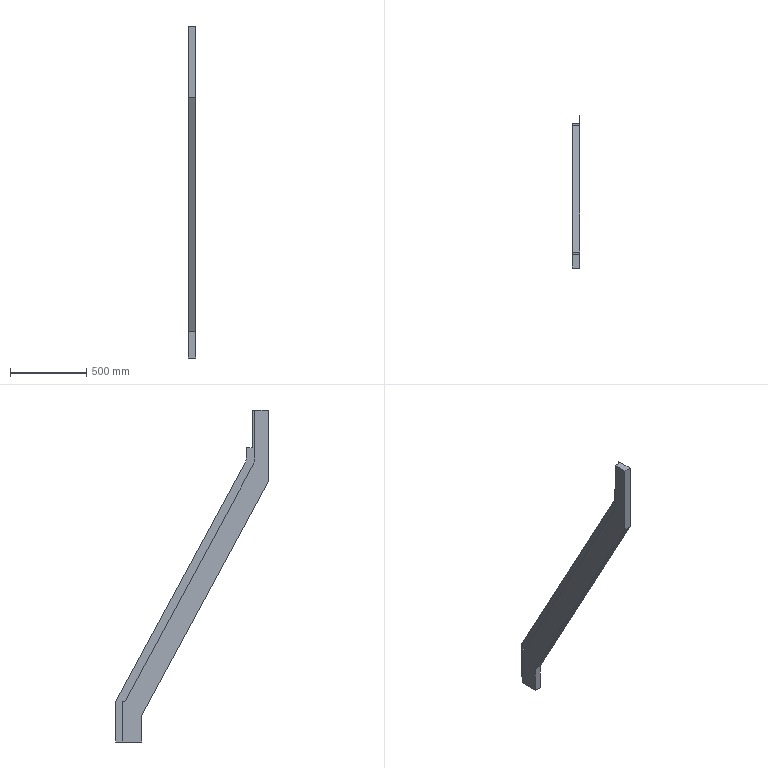Part | NX | 1 solid | 19 faces | box 48 x 1000 x 2173 mm | volume 15101075 mm3 | plane 17 | cylinder 2 | commonest cylinder face diameters 120 x1 228 x1
STEP:
#1=CARTESIAN_POINT('',(38.874,311.682,323.798));
#2=VERTEX_POINT('',#1);
#3=CARTESIAN_POINT('',(38.874,311.682,589.52));
#4=VERTEX_POINT('',#3);
#5=CARTESIAN_POINT('',(38.874,311.682,323.798));
#6=DIRECTION('',(0.,0.,1.));
#7=VECTOR('',#6,1.);
#8=LINE('',#5,#7);
#9=EDGE_CURVE('',#2,#4,#8,.T.);
#10=ORIENTED_EDGE('',*,*,#9,.T.);
#11=CARTESIAN_POINT('',(40.674,311.682,589.52));
#12=VERTEX_POINT('',#11);
#13=CARTESIAN_POINT('',(38.874,311.682,589.52));
#14=DIRECTION('',(1.,0.,0.));
#15=VECTOR('',#14,1.);
#16=LINE('',#13,#15);
#17=EDGE_CURVE('',#4,#12,#16,.T.);
#18=ORIENTED_EDGE('',*,*,#17,.T.);
#19=CARTESIAN_POINT('',(40.674,311.682,323.798));
#20=VERTEX_POINT('',#19);
#21=CARTESIAN_POINT('',(40.674,311.682,323.798));
#22=DIRECTION('',(0.,0.,1.));
#23=VECTOR('',#22,1.);
#24=LINE('',#21,#23);
#25=EDGE_CURVE('',#20,#12,#24,.T.);
#26=ORIENTED_EDGE('',*,*,#25,.F.);
#27=CARTESIAN_POINT('',(40.674,311.682,323.798));
#28=DIRECTION('',(-1.,0.,0.));
#29=VECTOR('',#28,1.);
#30=LINE('',#27,#29);
#31=EDGE_CURVE('',#20,#2,#30,.T.);
#32=ORIENTED_EDGE('',*,*,#31,.T.);
#33=EDGE_LOOP('',(#10,#18,#26,#32));
#34=FACE_OUTER_BOUND('',#33,.T.);
#35=CARTESIAN_POINT('',(40.674,311.682,323.798));
#36=DIRECTION('',(0.,1.,0.));
#37=DIRECTION('',(0.,0.,1.));
#38=AXIS2_PLACEMENT_3D('',#35,#36,#37);
#39=PLANE('',#38);
#40=ADVANCED_FACE('',(#34),#39,.T.);
#41=CARTESIAN_POINT('',(40.674,-583.499,2251.086));
#42=VERTEX_POINT('',#41);
#43=CARTESIAN_POINT('',(40.674,-544.499,2251.086));
#44=VERTEX_POINT('',#43);
#45=CARTESIAN_POINT('',(40.674,-544.499,2251.086));
#46=DIRECTION('',(0.,1.,0.));
#47=VECTOR('',#46,1.);
#48=LINE('',#45,#47);
#49=EDGE_CURVE('',#42,#44,#48,.T.);
#50=ORIENTED_EDGE('',*,*,#49,.F.);
#51=CARTESIAN_POINT('',(40.674,-583.499,2497.086));
#52=VERTEX_POINT('',#51);
#53=CARTESIAN_POINT('',(40.674,-583.499,2497.086));
#54=DIRECTION('',(0.,0.,-1.));
#55=VECTOR('',#54,1.);
#56=LINE('',#53,#55);
#57=EDGE_CURVE('',#52,#42,#56,.T.);
#58=ORIENTED_EDGE('',*,*,#57,.F.);
#59=CARTESIAN_POINT('',(40.674,-688.499,2497.086));
#60=VERTEX_POINT('',#59);
#61=CARTESIAN_POINT('',(40.674,-598.499,2497.086));
#62=DIRECTION('',(0.,-1.,0.));
#63=VECTOR('',#62,1.);
#64=LINE('',#61,#63);
#65=EDGE_CURVE('',#52,#60,#64,.T.);
#66=ORIENTED_EDGE('',*,*,#65,.T.);
#67=CARTESIAN_POINT('',(40.674,-688.499,2029.086));
#68=VERTEX_POINT('',#67);
#69=CARTESIAN_POINT('',(40.674,-688.499,2497.086));
#70=DIRECTION('',(0.,0.,-1.));
#71=VECTOR('',#70,1.);
#72=LINE('',#69,#71);
#73=EDGE_CURVE('',#60,#68,#72,.T.);
#74=ORIENTED_EDGE('',*,*,#73,.T.);
#75=CARTESIAN_POINT('',(40.674,141.389,497.262));
#76=VERTEX_POINT('',#75);
#77=CARTESIAN_POINT('',(40.674,141.389,497.262));
#78=DIRECTION('',(0.,0.4763,-0.8793));
#79=VECTOR('',#78,1.);
#80=LINE('',#77,#79);
#81=EDGE_CURVE('',#68,#76,#80,.T.);
#82=ORIENTED_EDGE('',*,*,#81,.T.);
#83=CARTESIAN_POINT('',(40.674,141.389,323.798));
#84=VERTEX_POINT('',#83);
#85=CARTESIAN_POINT('',(40.674,141.389,323.798));
#86=DIRECTION('',(0.,0.,1.));
#87=VECTOR('',#86,1.);
#88=LINE('',#85,#87);
#89=EDGE_CURVE('',#84,#76,#88,.T.);
#90=ORIENTED_EDGE('',*,*,#89,.F.);
#91=CARTESIAN_POINT('',(40.674,141.389,323.798));
#92=DIRECTION('',(0.,1.,0.));
#93=VECTOR('',#92,1.);
#94=LINE('',#91,#93);
#95=EDGE_CURVE('',#84,#20,#94,.T.);
#96=ORIENTED_EDGE('',*,*,#95,.T.);
#97=ORIENTED_EDGE('',*,*,#25,.T.);
#98=CARTESIAN_POINT('',(40.674,-537.255,2156.505));
#99=VERTEX_POINT('',#98);
#100=CARTESIAN_POINT('',(40.674,311.682,589.52));
#101=DIRECTION('',(0.,0.4763,-0.8793));
#102=VECTOR('',#101,1.);
#103=LINE('',#100,#102);
#104=EDGE_CURVE('',#99,#12,#103,.T.);
#105=ORIENTED_EDGE('',*,*,#104,.F.);
#106=CARTESIAN_POINT('',(40.674,-544.499,2185.086));
#107=VERTEX_POINT('',#106);
#108=CARTESIAN_POINT('',(40.674,-484.499,2185.086));
#109=DIRECTION('',(1.,0.,0.));
#110=DIRECTION('',(0.,0.,1.));
#111=AXIS2_PLACEMENT_3D('',#108,#109,#110);
#112=CIRCLE('',#111,60.);
#113=EDGE_CURVE('',#107,#99,#112,.T.);
#114=ORIENTED_EDGE('',*,*,#113,.F.);
#115=CARTESIAN_POINT('',(40.674,-544.499,2185.086));
#116=DIRECTION('',(0.,0.,-1.));
#117=VECTOR('',#116,1.);
#118=LINE('',#115,#117);
#119=EDGE_CURVE('',#44,#107,#118,.T.);
#120=ORIENTED_EDGE('',*,*,#119,.F.);
#121=EDGE_LOOP('',(#50,#58,#66,#74,#82,#90,#96,#97,#105,#114,#120));
#122=FACE_OUTER_BOUND('',#121,.T.);
#123=CARTESIAN_POINT('',(40.674,141.389,323.798));
#124=DIRECTION('',(1.,0.,0.));
#125=DIRECTION('',(0.,0.,-1.));
#126=AXIS2_PLACEMENT_3D('',#123,#124,#125);
#127=PLANE('',#126);
#128=ADVANCED_FACE('',(#122),#127,.T.);
#129=CARTESIAN_POINT('',(-7.326,141.389,497.262));
#130=VERTEX_POINT('',#129);
#131=CARTESIAN_POINT('',(-7.326,141.389,497.262));
#132=DIRECTION('',(1.,0.,0.));
#133=VECTOR('',#132,1.);
#134=LINE('',#131,#133);
#135=EDGE_CURVE('',#130,#76,#134,.T.);
#136=ORIENTED_EDGE('',*,*,#135,.F.);
#137=CARTESIAN_POINT('',(-7.326,141.389,323.798));
#138=VERTEX_POINT('',#137);
#139=CARTESIAN_POINT('',(-7.326,141.389,323.798));
#140=DIRECTION('',(0.,0.,1.));
#141=VECTOR('',#140,1.);
#142=LINE('',#139,#141);
#143=EDGE_CURVE('',#138,#130,#142,.T.);
#144=ORIENTED_EDGE('',*,*,#143,.F.);
#145=CARTESIAN_POINT('',(-7.326,141.389,323.798));
#146=DIRECTION('',(1.,0.,0.));
#147=VECTOR('',#146,1.);
#148=LINE('',#145,#147);
#149=EDGE_CURVE('',#138,#84,#148,.T.);
#150=ORIENTED_EDGE('',*,*,#149,.T.);
#151=ORIENTED_EDGE('',*,*,#89,.T.);
#152=EDGE_LOOP('',(#136,#144,#150,#151));
#153=FACE_OUTER_BOUND('',#152,.T.);
#154=CARTESIAN_POINT('',(-7.326,141.389,323.798));
#155=DIRECTION('',(0.,-1.,0.));
#156=DIRECTION('',(0.,0.,-1.));
#157=AXIS2_PLACEMENT_3D('',#154,#155,#156);
#158=PLANE('',#157);
#159=ADVANCED_FACE('',(#153),#158,.T.);
#160=ORIENTED_EDGE('',*,*,#143,.T.);
#161=CARTESIAN_POINT('',(-7.326,-688.499,2029.086));
#162=VERTEX_POINT('',#161);
#163=CARTESIAN_POINT('',(-7.326,141.389,497.262));
#164=DIRECTION('',(0.,0.4763,-0.8793));
#165=VECTOR('',#164,1.);
#166=LINE('',#163,#165);
#167=EDGE_CURVE('',#162,#130,#166,.T.);
#168=ORIENTED_EDGE('',*,*,#167,.F.);
#169=CARTESIAN_POINT('',(-7.326,-688.499,2497.086));
#170=VERTEX_POINT('',#169);
#171=CARTESIAN_POINT('',(-7.326,-688.499,2497.086));
#172=DIRECTION('',(0.,0.,-1.));
#173=VECTOR('',#172,1.);
#174=LINE('',#171,#173);
#175=EDGE_CURVE('',#170,#162,#174,.T.);
#176=ORIENTED_EDGE('',*,*,#175,.F.);
#177=CARTESIAN_POINT('',(-7.326,-598.499,2497.086));
#178=VERTEX_POINT('',#177);
#179=CARTESIAN_POINT('',(-7.326,-598.499,2497.086));
#180=DIRECTION('',(0.,-1.,0.));
#181=VECTOR('',#180,1.);
#182=LINE('',#179,#181);
#183=EDGE_CURVE('',#178,#170,#182,.T.);
#184=ORIENTED_EDGE('',*,*,#183,.F.);
#185=CARTESIAN_POINT('',(-7.326,-598.499,2185.086));
#186=VERTEX_POINT('',#185);
#187=CARTESIAN_POINT('',(-7.326,-598.499,2497.086));
#188=DIRECTION('',(0.,0.,1.));
#189=VECTOR('',#188,1.);
#190=LINE('',#187,#189);
#191=EDGE_CURVE('',#186,#178,#190,.T.);
#192=ORIENTED_EDGE('',*,*,#191,.F.);
#193=CARTESIAN_POINT('',(-7.326,-584.734,2130.782));
#194=VERTEX_POINT('',#193);
#195=CARTESIAN_POINT('',(-7.326,-484.499,2185.086));
#196=DIRECTION('',(-1.,0.,0.));
#197=DIRECTION('',(0.,0.,-1.));
#198=AXIS2_PLACEMENT_3D('',#195,#196,#197);
#199=CIRCLE('',#198,114.);
#200=EDGE_CURVE('',#194,#186,#199,.T.);
#201=ORIENTED_EDGE('',*,*,#200,.F.);
#202=CARTESIAN_POINT('',(-7.326,250.267,589.52));
#203=VERTEX_POINT('',#202);
#204=CARTESIAN_POINT('',(-7.326,-584.734,2130.782));
#205=DIRECTION('',(0.,-0.4763,0.8793));
#206=VECTOR('',#205,1.);
#207=LINE('',#204,#206);
#208=EDGE_CURVE('',#203,#194,#207,.T.);
#209=ORIENTED_EDGE('',*,*,#208,.F.);
#210=CARTESIAN_POINT('',(-7.326,264.202,589.52));
#211=VERTEX_POINT('',#210);
#212=CARTESIAN_POINT('',(-7.326,264.202,589.52));
#213=DIRECTION('',(0.,-1.,0.));
#214=VECTOR('',#213,1.);
#215=LINE('',#212,#214);
#216=EDGE_CURVE('',#211,#203,#215,.T.);
#217=ORIENTED_EDGE('',*,*,#216,.F.);
#218=CARTESIAN_POINT('',(-7.326,264.202,323.798));
#219=VERTEX_POINT('',#218);
#220=CARTESIAN_POINT('',(-7.326,264.202,323.798));
#221=DIRECTION('',(0.,0.,1.));
#222=VECTOR('',#221,1.);
#223=LINE('',#220,#222);
#224=EDGE_CURVE('',#219,#211,#223,.T.);
#225=ORIENTED_EDGE('',*,*,#224,.F.);
#226=CARTESIAN_POINT('',(-7.326,264.202,323.798));
#227=DIRECTION('',(0.,-1.,0.));
#228=VECTOR('',#227,1.);
#229=LINE('',#226,#228);
#230=EDGE_CURVE('',#219,#138,#229,.T.);
#231=ORIENTED_EDGE('',*,*,#230,.T.);
#232=EDGE_LOOP('',(#160,#168,#176,#184,#192,#201,#209,#217,#225,#231));
#233=FACE_OUTER_BOUND('',#232,.T.);
#234=CARTESIAN_POINT('',(-7.326,264.202,323.798));
#235=DIRECTION('',(-1.,0.,0.));
#236=DIRECTION('',(0.,0.,1.));
#237=AXIS2_PLACEMENT_3D('',#234,#235,#236);
#238=PLANE('',#237);
#239=ADVANCED_FACE('',(#233),#238,.T.);
#240=ORIENTED_EDGE('',*,*,#224,.T.);
#241=CARTESIAN_POINT('',(38.874,264.202,589.52));
#242=VERTEX_POINT('',#241);
#243=CARTESIAN_POINT('',(38.874,264.202,589.52));
#244=DIRECTION('',(-1.,0.,0.));
#245=VECTOR('',#244,1.);
#246=LINE('',#243,#245);
#247=EDGE_CURVE('',#242,#211,#246,.T.);
#248=ORIENTED_EDGE('',*,*,#247,.F.);
#249=CARTESIAN_POINT('',(38.874,264.202,323.798));
#250=VERTEX_POINT('',#249);
#251=CARTESIAN_POINT('',(38.874,264.202,323.798));
#252=DIRECTION('',(0.,0.,1.));
#253=VECTOR('',#252,1.);
#254=LINE('',#251,#253);
#255=EDGE_CURVE('',#250,#242,#254,.T.);
#256=ORIENTED_EDGE('',*,*,#255,.F.);
#257=CARTESIAN_POINT('',(38.874,264.202,323.798));
#258=DIRECTION('',(-1.,0.,0.));
#259=VECTOR('',#258,1.);
#260=LINE('',#257,#259);
#261=EDGE_CURVE('',#250,#219,#260,.T.);
#262=ORIENTED_EDGE('',*,*,#261,.T.);
#263=EDGE_LOOP('',(#240,#248,#256,#262));
#264=FACE_OUTER_BOUND('',#263,.T.);
#265=CARTESIAN_POINT('',(38.874,264.202,323.798));
#266=DIRECTION('',(0.,1.,0.));
#267=DIRECTION('',(0.,0.,1.));
#268=AXIS2_PLACEMENT_3D('',#265,#266,#267);
#269=PLANE('',#268);
#270=ADVANCED_FACE('',(#264),#269,.T.);
#271=CARTESIAN_POINT('',(38.874,-544.499,2251.086));
#272=VERTEX_POINT('',#271);
#273=CARTESIAN_POINT('',(38.874,-583.499,2251.086));
#274=VERTEX_POINT('',#273);
#275=CARTESIAN_POINT('',(38.874,311.682,2251.086));
#276=DIRECTION('',(0.,-1.,0.));
#277=VECTOR('',#276,1.);
#278=LINE('',#275,#277);
#279=EDGE_CURVE('',#272,#274,#278,.T.);
#280=ORIENTED_EDGE('',*,*,#279,.F.);
#281=CARTESIAN_POINT('',(38.874,-544.499,2185.086));
#282=VERTEX_POINT('',#281);
#283=CARTESIAN_POINT('',(38.874,-544.499,2185.086));
#284=DIRECTION('',(0.,0.,-1.));
#285=VECTOR('',#284,1.);
#286=LINE('',#283,#285);
#287=EDGE_CURVE('',#272,#282,#286,.T.);
#288=ORIENTED_EDGE('',*,*,#287,.T.);
#289=CARTESIAN_POINT('',(38.874,-537.255,2156.505));
#290=VERTEX_POINT('',#289);
#291=CARTESIAN_POINT('',(38.874,-484.499,2185.086));
#292=DIRECTION('',(1.,0.,0.));
#293=DIRECTION('',(0.,0.,1.));
#294=AXIS2_PLACEMENT_3D('',#291,#292,#293);
#295=CIRCLE('',#294,60.);
#296=EDGE_CURVE('',#282,#290,#295,.T.);
#297=ORIENTED_EDGE('',*,*,#296,.T.);
#298=CARTESIAN_POINT('',(38.874,311.682,589.52));
#299=DIRECTION('',(0.,0.4763,-0.8793));
#300=VECTOR('',#299,1.);
#301=LINE('',#298,#300);
#302=EDGE_CURVE('',#290,#4,#301,.T.);
#303=ORIENTED_EDGE('',*,*,#302,.T.);
#304=ORIENTED_EDGE('',*,*,#9,.F.);
#305=CARTESIAN_POINT('',(38.874,311.682,323.798));
#306=DIRECTION('',(0.,-1.,0.));
#307=VECTOR('',#306,1.);
#308=LINE('',#305,#307);
#309=EDGE_CURVE('',#2,#250,#308,.T.);
#310=ORIENTED_EDGE('',*,*,#309,.T.);
#311=ORIENTED_EDGE('',*,*,#255,.T.);
#312=CARTESIAN_POINT('',(38.874,250.267,589.52));
#313=VERTEX_POINT('',#312);
#314=CARTESIAN_POINT('',(38.874,311.682,589.52));
#315=DIRECTION('',(0.,-1.,0.));
#316=VECTOR('',#315,1.);
#317=LINE('',#314,#316);
#318=EDGE_CURVE('',#242,#313,#317,.T.);
#319=ORIENTED_EDGE('',*,*,#318,.T.);
#320=CARTESIAN_POINT('',(38.874,-584.734,2130.782));
#321=VERTEX_POINT('',#320);
#322=CARTESIAN_POINT('',(38.874,264.202,563.798));
#323=DIRECTION('',(0.,-0.4763,0.8793));
#324=VECTOR('',#323,1.);
#325=LINE('',#322,#324);
#326=EDGE_CURVE('',#313,#321,#325,.T.);
#327=ORIENTED_EDGE('',*,*,#326,.T.);
#328=CARTESIAN_POINT('',(38.874,-598.499,2185.086));
#329=VERTEX_POINT('',#328);
#330=CARTESIAN_POINT('',(38.874,-484.499,2185.086));
#331=DIRECTION('',(-1.,0.,0.));
#332=DIRECTION('',(0.,0.,1.));
#333=AXIS2_PLACEMENT_3D('',#330,#331,#332);
#334=CIRCLE('',#333,114.);
#335=EDGE_CURVE('',#321,#329,#334,.T.);
#336=ORIENTED_EDGE('',*,*,#335,.T.);
#337=CARTESIAN_POINT('',(38.874,-598.499,2497.086));
#338=VERTEX_POINT('',#337);
#339=CARTESIAN_POINT('',(38.874,-598.499,2185.086));
#340=DIRECTION('',(0.,0.,1.));
#341=VECTOR('',#340,1.);
#342=LINE('',#339,#341);
#343=EDGE_CURVE('',#329,#338,#342,.T.);
#344=ORIENTED_EDGE('',*,*,#343,.T.);
#345=CARTESIAN_POINT('',(38.874,-583.499,2497.086));
#346=VERTEX_POINT('',#345);
#347=CARTESIAN_POINT('',(38.874,-598.499,2497.086));
#348=DIRECTION('',(0.,1.,0.));
#349=VECTOR('',#348,1.);
#350=LINE('',#347,#349);
#351=EDGE_CURVE('',#338,#346,#350,.T.);
#352=ORIENTED_EDGE('',*,*,#351,.T.);
#353=CARTESIAN_POINT('',(38.874,-583.499,323.798));
#354=DIRECTION('',(0.,0.,1.));
#355=VECTOR('',#354,1.);
#356=LINE('',#353,#355);
#357=EDGE_CURVE('',#274,#346,#356,.T.);
#358=ORIENTED_EDGE('',*,*,#357,.F.);
#359=EDGE_LOOP('',(#280,#288,#297,#303,#304,#310,#311,#319,#327,#336,#344,#352,#358));
#360=FACE_OUTER_BOUND('',#359,.T.);
#361=CARTESIAN_POINT('',(38.874,311.682,323.798));
#362=DIRECTION('',(-1.,0.,0.));
#363=DIRECTION('',(0.,0.,1.));
#364=AXIS2_PLACEMENT_3D('',#361,#362,#363);
#365=PLANE('',#364);
#366=ADVANCED_FACE('',(#360),#365,.T.);
#367=ORIENTED_EDGE('',*,*,#31,.F.);
#368=ORIENTED_EDGE('',*,*,#95,.F.);
#369=ORIENTED_EDGE('',*,*,#149,.F.);
#370=ORIENTED_EDGE('',*,*,#230,.F.);
#371=ORIENTED_EDGE('',*,*,#261,.F.);
#372=ORIENTED_EDGE('',*,*,#309,.F.);
#373=EDGE_LOOP('',(#367,#368,#369,#370,#371,#372));
#374=FACE_OUTER_BOUND('',#373,.T.);
#375=CARTESIAN_POINT('',(38.874,311.682,323.798));
#376=DIRECTION('',(0.,0.,1.));
#377=DIRECTION('',(1.,0.,0.));
#378=AXIS2_PLACEMENT_3D('',#375,#376,#377);
#379=PLANE('',#378);
#380=ADVANCED_FACE('',(#374),#379,.F.);
#381=CARTESIAN_POINT('',(38.874,250.267,589.52));
#382=DIRECTION('',(-1.,0.,0.));
#383=VECTOR('',#382,1.);
#384=LINE('',#381,#383);
#385=EDGE_CURVE('',#313,#203,#384,.T.);
#386=ORIENTED_EDGE('',*,*,#385,.F.);
#387=ORIENTED_EDGE('',*,*,#318,.F.);
#388=ORIENTED_EDGE('',*,*,#247,.T.);
#389=ORIENTED_EDGE('',*,*,#216,.T.);
#390=EDGE_LOOP('',(#386,#387,#388,#389));
#391=FACE_OUTER_BOUND('',#390,.T.);
#392=CARTESIAN_POINT('',(38.874,311.682,589.52));
#393=DIRECTION('',(0.,0.,1.));
#394=DIRECTION('',(1.,0.,0.));
#395=AXIS2_PLACEMENT_3D('',#392,#393,#394);
#396=PLANE('',#395);
#397=ADVANCED_FACE('',(#391),#396,.T.);
#398=CARTESIAN_POINT('',(34.674,-583.499,2497.086));
#399=DIRECTION('',(1.,0.,0.));
#400=VECTOR('',#399,1.);
#401=LINE('',#398,#400);
#402=EDGE_CURVE('',#346,#52,#401,.T.);
#403=ORIENTED_EDGE('',*,*,#402,.F.);
#404=ORIENTED_EDGE('',*,*,#351,.F.);
#405=CARTESIAN_POINT('',(-7.326,-598.499,2497.086));
#406=DIRECTION('',(1.,0.,0.));
#407=VECTOR('',#406,1.);
#408=LINE('',#405,#407);
#409=EDGE_CURVE('',#178,#338,#408,.T.);
#410=ORIENTED_EDGE('',*,*,#409,.F.);
#411=ORIENTED_EDGE('',*,*,#183,.T.);
#412=CARTESIAN_POINT('',(-7.326,-688.499,2497.086));
#413=DIRECTION('',(1.,0.,0.));
#414=VECTOR('',#413,1.);
#415=LINE('',#412,#414);
#416=EDGE_CURVE('',#170,#60,#415,.T.);
#417=ORIENTED_EDGE('',*,*,#416,.T.);
#418=ORIENTED_EDGE('',*,*,#65,.F.);
#419=EDGE_LOOP('',(#403,#404,#410,#411,#417,#418));
#420=FACE_OUTER_BOUND('',#419,.T.);
#421=CARTESIAN_POINT('',(-7.326,-598.499,2497.086));
#422=DIRECTION('',(0.,0.,1.));
#423=DIRECTION('',(0.,-1.,0.));
#424=AXIS2_PLACEMENT_3D('',#421,#422,#423);
#425=PLANE('',#424);
#426=ADVANCED_FACE('',(#420),#425,.T.);
#427=ORIENTED_EDGE('',*,*,#343,.F.);
#428=CARTESIAN_POINT('',(-7.326,-598.499,2185.086));
#429=DIRECTION('',(1.,0.,0.));
#430=VECTOR('',#429,1.);
#431=LINE('',#428,#430);
#432=EDGE_CURVE('',#186,#329,#431,.T.);
#433=ORIENTED_EDGE('',*,*,#432,.F.);
#434=ORIENTED_EDGE('',*,*,#191,.T.);
#435=ORIENTED_EDGE('',*,*,#409,.T.);
#436=EDGE_LOOP('',(#427,#433,#434,#435));
#437=FACE_OUTER_BOUND('',#436,.T.);
#438=CARTESIAN_POINT('',(-7.326,-598.499,2497.086));
#439=DIRECTION('',(0.,1.,0.));
#440=DIRECTION('',(0.,0.,1.));
#441=AXIS2_PLACEMENT_3D('',#438,#439,#440);
#442=PLANE('',#441);
#443=ADVANCED_FACE('',(#437),#442,.T.);
#444=ORIENTED_EDGE('',*,*,#335,.F.);
#445=CARTESIAN_POINT('',(-7.326,-584.734,2130.782));
#446=DIRECTION('',(1.,0.,0.));
#447=VECTOR('',#446,1.);
#448=LINE('',#445,#447);
#449=EDGE_CURVE('',#194,#321,#448,.T.);
#450=ORIENTED_EDGE('',*,*,#449,.F.);
#451=ORIENTED_EDGE('',*,*,#200,.T.);
#452=ORIENTED_EDGE('',*,*,#432,.T.);
#453=EDGE_LOOP('',(#444,#450,#451,#452));
#454=FACE_OUTER_BOUND('',#453,.T.);
#455=CARTESIAN_POINT('',(-7.326,-484.499,2185.086));
#456=DIRECTION('',(1.,0.,0.));
#457=DIRECTION('',(0.,0.,-1.));
#458=AXIS2_PLACEMENT_3D('',#455,#456,#457);
#459=CYLINDRICAL_SURFACE('',#458,114.);
#460=ADVANCED_FACE('',(#454),#459,.F.);
#461=ORIENTED_EDGE('',*,*,#326,.F.);
#462=ORIENTED_EDGE('',*,*,#385,.T.);
#463=ORIENTED_EDGE('',*,*,#208,.T.);
#464=ORIENTED_EDGE('',*,*,#449,.T.);
#465=EDGE_LOOP('',(#461,#462,#463,#464));
#466=FACE_OUTER_BOUND('',#465,.T.);
#467=CARTESIAN_POINT('',(-7.326,-584.734,2130.782));
#468=DIRECTION('',(0.,0.8793,0.4763));
#469=DIRECTION('',(0.,-0.4763,0.8793));
#470=AXIS2_PLACEMENT_3D('',#467,#468,#469);
#471=PLANE('',#470);
#472=ADVANCED_FACE('',(#466),#471,.T.);
#473=ORIENTED_EDGE('',*,*,#81,.F.);
#474=CARTESIAN_POINT('',(-7.326,-688.499,2029.086));
#475=DIRECTION('',(1.,0.,0.));
#476=VECTOR('',#475,1.);
#477=LINE('',#474,#476);
#478=EDGE_CURVE('',#162,#68,#477,.T.);
#479=ORIENTED_EDGE('',*,*,#478,.F.);
#480=ORIENTED_EDGE('',*,*,#167,.T.);
#481=ORIENTED_EDGE('',*,*,#135,.T.);
#482=EDGE_LOOP('',(#473,#479,#480,#481));
#483=FACE_OUTER_BOUND('',#482,.T.);
#484=CARTESIAN_POINT('',(-7.326,141.389,497.262));
#485=DIRECTION('',(0.,-0.8793,-0.4763));
#486=DIRECTION('',(0.,0.4763,-0.8793));
#487=AXIS2_PLACEMENT_3D('',#484,#485,#486);
#488=PLANE('',#487);
#489=ADVANCED_FACE('',(#483),#488,.T.);
#490=ORIENTED_EDGE('',*,*,#73,.F.);
#491=ORIENTED_EDGE('',*,*,#416,.F.);
#492=ORIENTED_EDGE('',*,*,#175,.T.);
#493=ORIENTED_EDGE('',*,*,#478,.T.);
#494=EDGE_LOOP('',(#490,#491,#492,#493));
#495=FACE_OUTER_BOUND('',#494,.T.);
#496=CARTESIAN_POINT('',(-7.326,-688.499,2497.086));
#497=DIRECTION('',(0.,-1.,0.));
#498=DIRECTION('',(0.,0.,-1.));
#499=AXIS2_PLACEMENT_3D('',#496,#497,#498);
#500=PLANE('',#499);
#501=ADVANCED_FACE('',(#495),#500,.T.);
#502=ORIENTED_EDGE('',*,*,#287,.F.);
#503=CARTESIAN_POINT('',(38.874,-544.499,2251.086));
#504=DIRECTION('',(1.,0.,0.));
#505=VECTOR('',#504,1.);
#506=LINE('',#503,#505);
#507=EDGE_CURVE('',#272,#44,#506,.T.);
#508=ORIENTED_EDGE('',*,*,#507,.T.);
#509=ORIENTED_EDGE('',*,*,#119,.T.);
#510=CARTESIAN_POINT('',(38.874,-544.499,2185.086));
#511=DIRECTION('',(1.,0.,0.));
#512=VECTOR('',#511,1.);
#513=LINE('',#510,#512);
#514=EDGE_CURVE('',#282,#107,#513,.T.);
#515=ORIENTED_EDGE('',*,*,#514,.F.);
#516=EDGE_LOOP('',(#502,#508,#509,#515));
#517=FACE_OUTER_BOUND('',#516,.T.);
#518=CARTESIAN_POINT('',(38.874,-544.499,2185.086));
#519=DIRECTION('',(0.,-1.,0.));
#520=DIRECTION('',(0.,0.,-1.));
#521=AXIS2_PLACEMENT_3D('',#518,#519,#520);
#522=PLANE('',#521);
#523=ADVANCED_FACE('',(#517),#522,.F.);
#524=ORIENTED_EDGE('',*,*,#113,.T.);
#525=CARTESIAN_POINT('',(38.874,-537.255,2156.505));
#526=DIRECTION('',(1.,0.,0.));
#527=VECTOR('',#526,1.);
#528=LINE('',#525,#527);
#529=EDGE_CURVE('',#290,#99,#528,.T.);
#530=ORIENTED_EDGE('',*,*,#529,.F.);
#531=ORIENTED_EDGE('',*,*,#296,.F.);
#532=ORIENTED_EDGE('',*,*,#514,.T.);
#533=EDGE_LOOP('',(#524,#530,#531,#532));
#534=FACE_OUTER_BOUND('',#533,.T.);
#535=CARTESIAN_POINT('',(38.874,-484.499,2185.086));
#536=DIRECTION('',(1.,0.,0.));
#537=DIRECTION('',(0.,0.,-1.));
#538=AXIS2_PLACEMENT_3D('',#535,#536,#537);
#539=CYLINDRICAL_SURFACE('',#538,60.);
#540=ADVANCED_FACE('',(#534),#539,.F.);
#541=ORIENTED_EDGE('',*,*,#104,.T.);
#542=ORIENTED_EDGE('',*,*,#17,.F.);
#543=ORIENTED_EDGE('',*,*,#302,.F.);
#544=ORIENTED_EDGE('',*,*,#529,.T.);
#545=EDGE_LOOP('',(#541,#542,#543,#544));
#546=FACE_OUTER_BOUND('',#545,.T.);
#547=CARTESIAN_POINT('',(38.874,311.682,589.52));
#548=DIRECTION('',(0.,-0.8793,-0.4763));
#549=DIRECTION('',(0.,0.4763,-0.8793));
#550=AXIS2_PLACEMENT_3D('',#547,#548,#549);
#551=PLANE('',#550);
#552=ADVANCED_FACE('',(#546),#551,.F.);
#553=ORIENTED_EDGE('',*,*,#279,.T.);
#554=CARTESIAN_POINT('',(34.674,-583.499,2251.086));
#555=DIRECTION('',(1.,0.,0.));
#556=VECTOR('',#555,1.);
#557=LINE('',#554,#556);
#558=EDGE_CURVE('',#274,#42,#557,.T.);
#559=ORIENTED_EDGE('',*,*,#558,.T.);
#560=ORIENTED_EDGE('',*,*,#49,.T.);
#561=ORIENTED_EDGE('',*,*,#507,.F.);
#562=EDGE_LOOP('',(#553,#559,#560,#561));
#563=FACE_OUTER_BOUND('',#562,.T.);
#564=CARTESIAN_POINT('',(34.674,-544.499,2251.086));
#565=DIRECTION('',(0.,0.,-1.));
#566=DIRECTION('',(-1.,0.,0.));
#567=AXIS2_PLACEMENT_3D('',#564,#565,#566);
#568=PLANE('',#567);
#569=ADVANCED_FACE('',(#563),#568,.F.);
#570=ORIENTED_EDGE('',*,*,#357,.T.);
#571=ORIENTED_EDGE('',*,*,#402,.T.);
#572=ORIENTED_EDGE('',*,*,#57,.T.);
#573=ORIENTED_EDGE('',*,*,#558,.F.);
#574=EDGE_LOOP('',(#570,#571,#572,#573));
#575=FACE_OUTER_BOUND('',#574,.T.);
#576=CARTESIAN_POINT('',(34.674,-583.499,2497.086));
#577=DIRECTION('',(0.,-1.,0.));
#578=DIRECTION('',(0.,0.,-1.));
#579=AXIS2_PLACEMENT_3D('',#576,#577,#578);
#580=PLANE('',#579);
#581=ADVANCED_FACE('',(#575),#580,.F.);
#582=CLOSED_SHELL('',(#40,#128,#159,#239,#270,#366,#380,#397,#426,#443,#460,#472,#489,#501,#523,#540,#552,#569,#581));
#583=MANIFOLD_SOLID_BREP('',#582);
#584=(LENGTH_UNIT()NAMED_UNIT(*)SI_UNIT(.MILLI.,.METRE.));
#585=UNCERTAINTY_MEASURE_WITH_UNIT(LENGTH_MEASURE(0.00002),#584,'','');
#586=(NAMED_UNIT(*)PLANE_ANGLE_UNIT()SI_UNIT($,.RADIAN.));
#587=PLANE_ANGLE_MEASURE_WITH_UNIT(PLANE_ANGLE_MEASURE(0.01745),#586);
#588=DIMENSIONAL_EXPONENTS(0.,0.,0.,0.,0.,0.,0.);
#589=(CONVERSION_BASED_UNIT('DEGREE',#587)NAMED_UNIT(#588)PLANE_ANGLE_UNIT());
#590=(NAMED_UNIT(*)SI_UNIT($,.STERADIAN.)SOLID_ANGLE_UNIT());
#591=(GEOMETRIC_REPRESENTATION_CONTEXT(3)GLOBAL_UNCERTAINTY_ASSIGNED_CONTEXT((#585))GLOBAL_UNIT_ASSIGNED_CONTEXT((#584,#589,#590))REPRESENTATION_CONTEXT('',''));
#592=ADVANCED_BREP_SHAPE_REPRESENTATION('',(#583),#591);